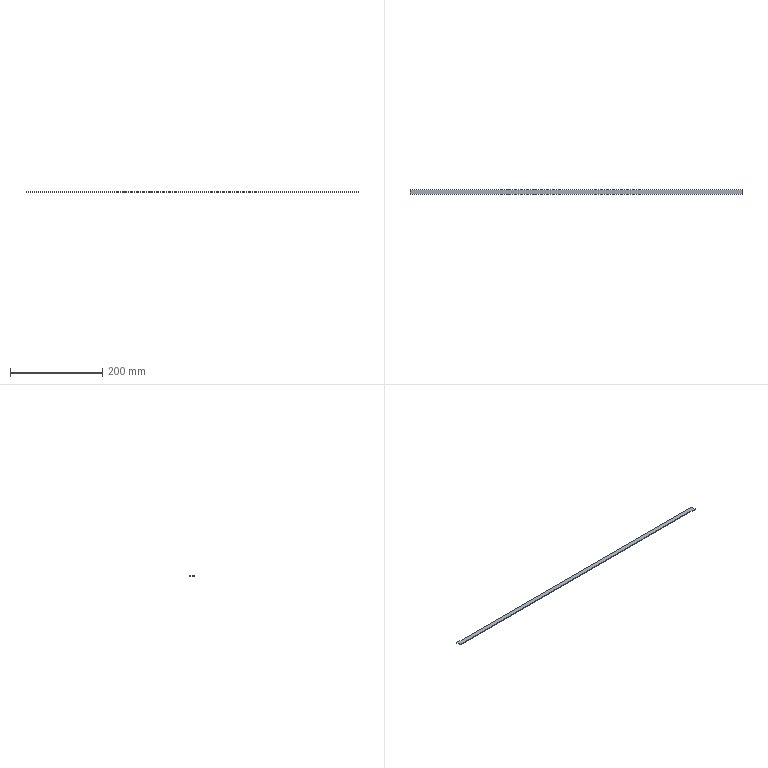Part | STEP file | BODY22_E-RAM6-S-640-ME30-C5 | 1 solid | 6 faces | box 720 x 10 x 1.5 mm | volume 10800 mm3 | plane 6
STEP:
#1=CARTESIAN_POINT('',(-360.,5.,0.));
#2=VERTEX_POINT('',#1);
#3=CARTESIAN_POINT('',(-360.,-5.,0.));
#4=VERTEX_POINT('',#3);
#5=CARTESIAN_POINT('',(-360.,-5.,0.));
#6=DIRECTION('',(0.,-1.,0.));
#7=VECTOR('',#6,1000.);
#8=LINE('',#5,#7);
#9=EDGE_CURVE('',#2,#4,#8,.T.);
#10=ORIENTED_EDGE('',*,*,#9,.T.);
#11=CARTESIAN_POINT('',(-360.,-5.,1.5));
#12=VERTEX_POINT('',#11);
#13=CARTESIAN_POINT('',(-360.,-5.,1.5));
#14=DIRECTION('',(0.,0.,-1.));
#15=VECTOR('',#14,1000.);
#16=LINE('',#13,#15);
#17=EDGE_CURVE('',#12,#4,#16,.T.);
#18=ORIENTED_EDGE('',*,*,#17,.F.);
#19=CARTESIAN_POINT('',(-360.,5.,1.5));
#20=VERTEX_POINT('',#19);
#21=CARTESIAN_POINT('',(-360.,-5.,1.5));
#22=DIRECTION('',(0.,-1.,0.));
#23=VECTOR('',#22,1000.);
#24=LINE('',#21,#23);
#25=EDGE_CURVE('',#20,#12,#24,.T.);
#26=ORIENTED_EDGE('',*,*,#25,.F.);
#27=CARTESIAN_POINT('',(-360.,5.,1.5));
#28=DIRECTION('',(0.,0.,-1.));
#29=VECTOR('',#28,1000.);
#30=LINE('',#27,#29);
#31=EDGE_CURVE('',#20,#2,#30,.T.);
#32=ORIENTED_EDGE('',*,*,#31,.T.);
#33=EDGE_LOOP('',(#10,#18,#26,#32));
#34=FACE_OUTER_BOUND('',#33,.T.);
#35=CARTESIAN_POINT('',(-360.,-5.,1.5));
#36=DIRECTION('',(1.,0.,0.));
#37=DIRECTION('',(0.,0.,-1.));
#38=AXIS2_PLACEMENT_3D('',#35,#36,#37);
#39=PLANE('',#38);
#40=ADVANCED_FACE('',(#34),#39,.F.);
#41=CARTESIAN_POINT('',(360.,-5.,0.));
#42=VERTEX_POINT('',#41);
#43=CARTESIAN_POINT('',(360.,-5.,0.));
#44=DIRECTION('',(1.,0.,0.));
#45=VECTOR('',#44,1000.);
#46=LINE('',#43,#45);
#47=EDGE_CURVE('',#4,#42,#46,.T.);
#48=ORIENTED_EDGE('',*,*,#47,.T.);
#49=CARTESIAN_POINT('',(360.,-5.,1.5));
#50=VERTEX_POINT('',#49);
#51=CARTESIAN_POINT('',(360.,-5.,1.5));
#52=DIRECTION('',(0.,0.,-1.));
#53=VECTOR('',#52,1000.);
#54=LINE('',#51,#53);
#55=EDGE_CURVE('',#50,#42,#54,.T.);
#56=ORIENTED_EDGE('',*,*,#55,.F.);
#57=CARTESIAN_POINT('',(360.,-5.,1.5));
#58=DIRECTION('',(1.,0.,0.));
#59=VECTOR('',#58,1000.);
#60=LINE('',#57,#59);
#61=EDGE_CURVE('',#12,#50,#60,.T.);
#62=ORIENTED_EDGE('',*,*,#61,.F.);
#63=ORIENTED_EDGE('',*,*,#17,.T.);
#64=EDGE_LOOP('',(#48,#56,#62,#63));
#65=FACE_OUTER_BOUND('',#64,.T.);
#66=CARTESIAN_POINT('',(360.,-5.,1.5));
#67=DIRECTION('',(0.,1.,0.));
#68=DIRECTION('',(-1.,0.,0.));
#69=AXIS2_PLACEMENT_3D('',#66,#67,#68);
#70=PLANE('',#69);
#71=ADVANCED_FACE('',(#65),#70,.F.);
#72=CARTESIAN_POINT('',(360.,5.,0.));
#73=VERTEX_POINT('',#72);
#74=CARTESIAN_POINT('',(360.,-5.,0.));
#75=DIRECTION('',(0.,1.,0.));
#76=VECTOR('',#75,1000.);
#77=LINE('',#74,#76);
#78=EDGE_CURVE('',#42,#73,#77,.T.);
#79=ORIENTED_EDGE('',*,*,#78,.T.);
#80=CARTESIAN_POINT('',(360.,5.,1.5));
#81=VERTEX_POINT('',#80);
#82=CARTESIAN_POINT('',(360.,5.,1.5));
#83=DIRECTION('',(0.,0.,-1.));
#84=VECTOR('',#83,1000.);
#85=LINE('',#82,#84);
#86=EDGE_CURVE('',#81,#73,#85,.T.);
#87=ORIENTED_EDGE('',*,*,#86,.F.);
#88=CARTESIAN_POINT('',(360.,-5.,1.5));
#89=DIRECTION('',(0.,1.,0.));
#90=VECTOR('',#89,1000.);
#91=LINE('',#88,#90);
#92=EDGE_CURVE('',#50,#81,#91,.T.);
#93=ORIENTED_EDGE('',*,*,#92,.F.);
#94=ORIENTED_EDGE('',*,*,#55,.T.);
#95=EDGE_LOOP('',(#79,#87,#93,#94));
#96=FACE_OUTER_BOUND('',#95,.T.);
#97=CARTESIAN_POINT('',(360.,-5.,1.5));
#98=DIRECTION('',(-1.,0.,0.));
#99=DIRECTION('',(0.,0.,1.));
#100=AXIS2_PLACEMENT_3D('',#97,#98,#99);
#101=PLANE('',#100);
#102=ADVANCED_FACE('',(#96),#101,.F.);
#103=CARTESIAN_POINT('',(360.,5.,0.));
#104=DIRECTION('',(-1.,0.,0.));
#105=VECTOR('',#104,1000.);
#106=LINE('',#103,#105);
#107=EDGE_CURVE('',#73,#2,#106,.T.);
#108=ORIENTED_EDGE('',*,*,#107,.T.);
#109=ORIENTED_EDGE('',*,*,#31,.F.);
#110=CARTESIAN_POINT('',(360.,5.,1.5));
#111=DIRECTION('',(-1.,0.,0.));
#112=VECTOR('',#111,1000.);
#113=LINE('',#110,#112);
#114=EDGE_CURVE('',#81,#20,#113,.T.);
#115=ORIENTED_EDGE('',*,*,#114,.F.);
#116=ORIENTED_EDGE('',*,*,#86,.T.);
#117=EDGE_LOOP('',(#108,#109,#115,#116));
#118=FACE_OUTER_BOUND('',#117,.T.);
#119=CARTESIAN_POINT('',(360.,5.,1.5));
#120=DIRECTION('',(0.,-1.,0.));
#121=DIRECTION('',(1.,0.,0.));
#122=AXIS2_PLACEMENT_3D('',#119,#120,#121);
#123=PLANE('',#122);
#124=ADVANCED_FACE('',(#118),#123,.F.);
#125=ORIENTED_EDGE('',*,*,#25,.T.);
#126=ORIENTED_EDGE('',*,*,#61,.T.);
#127=ORIENTED_EDGE('',*,*,#92,.T.);
#128=ORIENTED_EDGE('',*,*,#114,.T.);
#129=EDGE_LOOP('',(#125,#126,#127,#128));
#130=FACE_OUTER_BOUND('',#129,.T.);
#131=CARTESIAN_POINT('',(0.,0.,1.5));
#132=DIRECTION('',(0.,0.,1.));
#133=DIRECTION('',(1.,0.,0.));
#134=AXIS2_PLACEMENT_3D('',#131,#132,#133);
#135=PLANE('',#134);
#136=ADVANCED_FACE('',(#130),#135,.T.);
#137=ORIENTED_EDGE('',*,*,#9,.F.);
#138=ORIENTED_EDGE('',*,*,#107,.F.);
#139=ORIENTED_EDGE('',*,*,#78,.F.);
#140=ORIENTED_EDGE('',*,*,#47,.F.);
#141=EDGE_LOOP('',(#137,#138,#139,#140));
#142=FACE_OUTER_BOUND('',#141,.T.);
#143=CARTESIAN_POINT('',(0.,0.,0.));
#144=DIRECTION('',(0.,0.,1.));
#145=DIRECTION('',(1.,0.,0.));
#146=AXIS2_PLACEMENT_3D('',#143,#144,#145);
#147=PLANE('',#146);
#148=ADVANCED_FACE('',(#142),#147,.F.);
#149=CLOSED_SHELL('',(#40,#71,#102,#124,#136,#148));
#150=MANIFOLD_SOLID_BREP('',#149);
#151=(LENGTH_UNIT()NAMED_UNIT(*)SI_UNIT(.MILLI.,.METRE.));
#152=UNCERTAINTY_MEASURE_WITH_UNIT(LENGTH_MEASURE(0.01),#151,'','');
#153=(NAMED_UNIT(*)PLANE_ANGLE_UNIT()SI_UNIT($,.RADIAN.));
#154=(NAMED_UNIT(*)SI_UNIT($,.STERADIAN.)SOLID_ANGLE_UNIT());
#155=(GEOMETRIC_REPRESENTATION_CONTEXT(3)GLOBAL_UNCERTAINTY_ASSIGNED_CONTEXT((#152))GLOBAL_UNIT_ASSIGNED_CONTEXT((#151,#153,#154))REPRESENTATION_CONTEXT('',''));
#156=ADVANCED_BREP_SHAPE_REPRESENTATION('',(#150),#155);